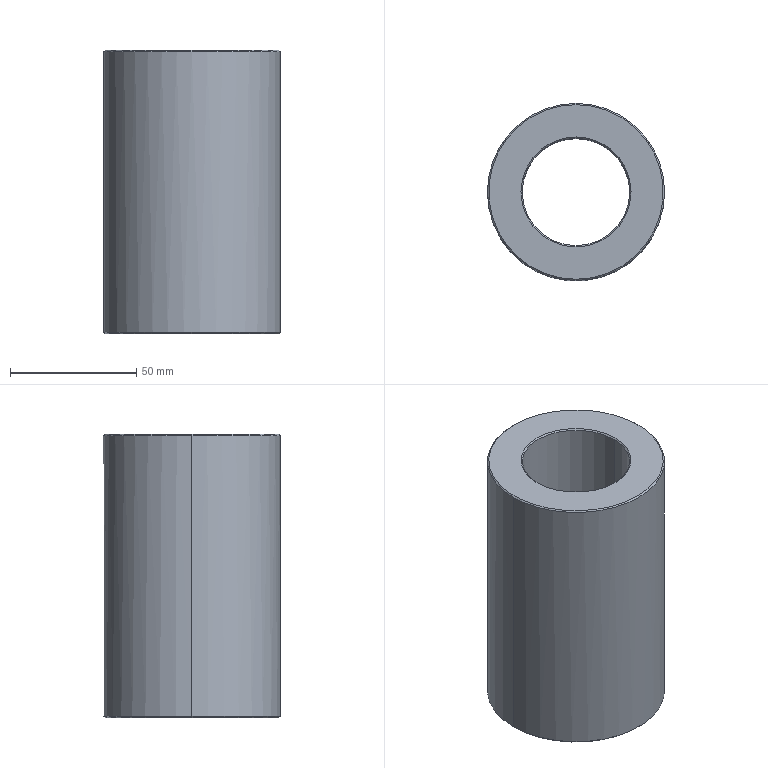Part | STEP file | Bearing sleeve_063_25.step_1 | 1 solid | 14 faces | box 70 x 70 x 112 mm | volume 272052 mm3 | cone 8 | cylinder 4 | plane 2 | commonest cylinder face diameters 42.5 x2 70 x2
STEP:
#1=CARTESIAN_POINT('',(0.,0.,0.));
#2=DIRECTION('',(0.,0.,1.));
#3=DIRECTION('',(1.,0.,0.));
#4=AXIS2_PLACEMENT_3D('',#1,#2,#3);
#5=CARTESIAN_POINT('',(35.,0.,-55.5));
#6=VERTEX_POINT('',#5);
#7=CARTESIAN_POINT('',(-35.,0.,-55.5));
#8=VERTEX_POINT('',#7);
#9=CARTESIAN_POINT('',(0.,0.,-55.5));
#10=DIRECTION('',(0.,0.,1.));
#11=DIRECTION('',(1.,0.,0.));
#12=AXIS2_PLACEMENT_3D('',#9,#10,#11);
#13=CIRCLE('',#12,35.);
#14=CARTESIAN_POINT('',(0.,0.,96.873));
#15=DIRECTION('',(0.,0.,1.));
#16=DIRECTION('',(1.,0.,0.));
#17=AXIS2_PLACEMENT_3D('',#14,#15,#16);
#18=CYLINDRICAL_SURFACE('',#17,35.);
#19=CARTESIAN_POINT('',(0.,-152.373));
#20=DIRECTION('',(1.,0.));
#21=VECTOR('',#20,1.);
#22=LINE('',#19,#21);
#23=(GEOMETRIC_REPRESENTATION_CONTEXT(2)PARAMETRIC_REPRESENTATION_CONTEXT()REPRESENTATION_CONTEXT('',''));
#24=DEFINITIONAL_REPRESENTATION('',(#22),#23);
#25=PCURVE('',#18,#24);
#26=CARTESIAN_POINT('',(0.,0.,-55.5));
#27=DIRECTION('',(0.,0.,1.));
#28=DIRECTION('',(1.,0.,0.));
#29=AXIS2_PLACEMENT_3D('',#26,#27,#28);
#30=CONICAL_SURFACE('',#29,35.,0.7854);
#31=CARTESIAN_POINT('',(0.,0.));
#32=DIRECTION('',(1.,0.));
#33=VECTOR('',#32,1.);
#34=LINE('',#31,#33);
#35=(GEOMETRIC_REPRESENTATION_CONTEXT(2)PARAMETRIC_REPRESENTATION_CONTEXT()REPRESENTATION_CONTEXT('',''));
#36=DEFINITIONAL_REPRESENTATION('',(#34),#35);
#37=PCURVE('',#30,#36);
#38=SURFACE_CURVE('',#13,(#25,#37),.PCURVE_S1.);
#39=EDGE_CURVE('',#6,#8,#38,.T.);
#40=ORIENTED_EDGE('',*,*,#39,.T.);
#41=CARTESIAN_POINT('',(-35.,0.,55.5));
#42=VERTEX_POINT('',#41);
#43=CARTESIAN_POINT('',(-35.,0.,96.873));
#44=DIRECTION('',(0.,0.,1.));
#45=VECTOR('',#44,1.);
#46=LINE('',#43,#45);
#47=CARTESIAN_POINT('',(3.142,0.));
#48=DIRECTION('',(0.,1.));
#49=VECTOR('',#48,1.);
#50=LINE('',#47,#49);
#51=(GEOMETRIC_REPRESENTATION_CONTEXT(2)PARAMETRIC_REPRESENTATION_CONTEXT()REPRESENTATION_CONTEXT('',''));
#52=DEFINITIONAL_REPRESENTATION('',(#50),#51);
#53=PCURVE('',#18,#52);
#54=CARTESIAN_POINT('',(0.,0.,96.873));
#55=DIRECTION('',(0.,0.,1.));
#56=DIRECTION('',(1.,0.,0.));
#57=AXIS2_PLACEMENT_3D('',#54,#55,#56);
#58=CYLINDRICAL_SURFACE('',#57,35.);
#59=CARTESIAN_POINT('',(3.142,0.));
#60=DIRECTION('',(0.,1.));
#61=VECTOR('',#60,1.);
#62=LINE('',#59,#61);
#63=(GEOMETRIC_REPRESENTATION_CONTEXT(2)PARAMETRIC_REPRESENTATION_CONTEXT()REPRESENTATION_CONTEXT('',''));
#64=DEFINITIONAL_REPRESENTATION('',(#62),#63);
#65=PCURVE('',#58,#64);
#66=SURFACE_CURVE('',#46,(#53,#65),.PCURVE_S1.);
#67=EDGE_CURVE('',#8,#42,#66,.T.);
#68=ORIENTED_EDGE('',*,*,#67,.T.);
#69=CARTESIAN_POINT('',(0.,35.,55.5));
#70=VERTEX_POINT('',#69);
#71=CARTESIAN_POINT('',(0.,0.,55.5));
#72=DIRECTION('',(0.,0.,-1.));
#73=DIRECTION('',(1.,0.,0.));
#74=AXIS2_PLACEMENT_3D('',#71,#72,#73);
#75=CIRCLE('',#74,35.);
#76=CARTESIAN_POINT('',(6.283,-41.373));
#77=DIRECTION('',(-1.,0.));
#78=VECTOR('',#77,1.);
#79=LINE('',#76,#78);
#80=(GEOMETRIC_REPRESENTATION_CONTEXT(2)PARAMETRIC_REPRESENTATION_CONTEXT()REPRESENTATION_CONTEXT('',''));
#81=DEFINITIONAL_REPRESENTATION('',(#79),#80);
#82=PCURVE('',#18,#81);
#83=CARTESIAN_POINT('',(0.,0.,55.5));
#84=DIRECTION('',(0.,0.,-1.));
#85=DIRECTION('',(0.,1.,0.));
#86=AXIS2_PLACEMENT_3D('',#83,#84,#85);
#87=CONICAL_SURFACE('',#86,35.,0.7854);
#88=CARTESIAN_POINT('',(1.571,0.));
#89=DIRECTION('',(1.,0.));
#90=VECTOR('',#89,1.);
#91=LINE('',#88,#90);
#92=(GEOMETRIC_REPRESENTATION_CONTEXT(2)PARAMETRIC_REPRESENTATION_CONTEXT()REPRESENTATION_CONTEXT('',''));
#93=DEFINITIONAL_REPRESENTATION('',(#91),#92);
#94=PCURVE('',#87,#93);
#95=SURFACE_CURVE('',#75,(#82,#94),.PCURVE_S1.);
#96=EDGE_CURVE('',#42,#70,#95,.T.);
#97=ORIENTED_EDGE('',*,*,#96,.T.);
#98=CARTESIAN_POINT('',(35.,0.,55.5));
#99=VERTEX_POINT('',#98);
#100=CARTESIAN_POINT('',(0.,0.,55.5));
#101=DIRECTION('',(0.,0.,-1.));
#102=DIRECTION('',(1.,0.,0.));
#103=AXIS2_PLACEMENT_3D('',#100,#101,#102);
#104=CIRCLE('',#103,35.);
#105=CARTESIAN_POINT('',(6.283,-41.373));
#106=DIRECTION('',(-1.,0.));
#107=VECTOR('',#106,1.);
#108=LINE('',#105,#107);
#109=(GEOMETRIC_REPRESENTATION_CONTEXT(2)PARAMETRIC_REPRESENTATION_CONTEXT()REPRESENTATION_CONTEXT('',''));
#110=DEFINITIONAL_REPRESENTATION('',(#108),#109);
#111=PCURVE('',#18,#110);
#112=CARTESIAN_POINT('',(0.,0.,55.5));
#113=DIRECTION('',(0.,0.,-1.));
#114=DIRECTION('',(0.,1.,0.));
#115=AXIS2_PLACEMENT_3D('',#112,#113,#114);
#116=CONICAL_SURFACE('',#115,35.,0.7854);
#117=CARTESIAN_POINT('',(-4.712,0.));
#118=DIRECTION('',(1.,0.));
#119=VECTOR('',#118,1.);
#120=LINE('',#117,#119);
#121=(GEOMETRIC_REPRESENTATION_CONTEXT(2)PARAMETRIC_REPRESENTATION_CONTEXT()REPRESENTATION_CONTEXT('',''));
#122=DEFINITIONAL_REPRESENTATION('',(#120),#121);
#123=PCURVE('',#116,#122);
#124=SURFACE_CURVE('',#104,(#111,#123),.PCURVE_S1.);
#125=EDGE_CURVE('',#70,#99,#124,.T.);
#126=ORIENTED_EDGE('',*,*,#125,.T.);
#127=CARTESIAN_POINT('',(35.,0.,96.873));
#128=DIRECTION('',(0.,0.,1.));
#129=VECTOR('',#128,1.);
#130=LINE('',#127,#129);
#131=CARTESIAN_POINT('',(0.,0.));
#132=DIRECTION('',(0.,1.));
#133=VECTOR('',#132,1.);
#134=LINE('',#131,#133);
#135=(GEOMETRIC_REPRESENTATION_CONTEXT(2)PARAMETRIC_REPRESENTATION_CONTEXT()REPRESENTATION_CONTEXT('',''));
#136=DEFINITIONAL_REPRESENTATION('',(#134),#135);
#137=PCURVE('',#18,#136);
#138=CARTESIAN_POINT('',(6.283,0.));
#139=DIRECTION('',(0.,1.));
#140=VECTOR('',#139,1.);
#141=LINE('',#138,#140);
#142=(GEOMETRIC_REPRESENTATION_CONTEXT(2)PARAMETRIC_REPRESENTATION_CONTEXT()REPRESENTATION_CONTEXT('',''));
#143=DEFINITIONAL_REPRESENTATION('',(#141),#142);
#144=PCURVE('',#58,#143);
#145=SURFACE_CURVE('',#130,(#137,#144),.PCURVE_S1.);
#146=EDGE_CURVE('',#6,#99,#145,.T.);
#147=ORIENTED_EDGE('',*,*,#146,.F.);
#148=EDGE_LOOP('',(#40,#68,#97,#126,#147));
#149=FACE_BOUND('',#148,.T.);
#150=ADVANCED_FACE('',(#149),#18,.T.);
#151=CARTESIAN_POINT('',(0.,34.5,56.));
#152=VERTEX_POINT('',#151);
#153=CARTESIAN_POINT('',(0.,-34.5,56.));
#154=VERTEX_POINT('',#153);
#155=CARTESIAN_POINT('',(0.,0.,56.));
#156=DIRECTION('',(0.,0.,-1.));
#157=DIRECTION('',(0.,1.,0.));
#158=AXIS2_PLACEMENT_3D('',#155,#156,#157);
#159=CIRCLE('',#158,34.5);
#160=CARTESIAN_POINT('',(0.,-0.5));
#161=DIRECTION('',(1.,0.));
#162=VECTOR('',#161,1.);
#163=LINE('',#160,#162);
#164=(GEOMETRIC_REPRESENTATION_CONTEXT(2)PARAMETRIC_REPRESENTATION_CONTEXT()REPRESENTATION_CONTEXT('',''));
#165=DEFINITIONAL_REPRESENTATION('',(#163),#164);
#166=PCURVE('',#116,#165);
#167=CARTESIAN_POINT('',(0.,21.75,56.));
#168=DIRECTION('',(0.,0.,-1.));
#169=DIRECTION('',(-1.,0.,0.));
#170=AXIS2_PLACEMENT_3D('',#167,#168,#169);
#171=PLANE('',#170);
#172=CARTESIAN_POINT('',(0.,-21.75));
#173=DIRECTION('',(0.,1.));
#174=AXIS2_PLACEMENT_2D('',#172,#173);
#175=CIRCLE('',#174,34.5);
#176=(GEOMETRIC_REPRESENTATION_CONTEXT(2)PARAMETRIC_REPRESENTATION_CONTEXT()REPRESENTATION_CONTEXT('',''));
#177=DEFINITIONAL_REPRESENTATION('',(#175),#176);
#178=PCURVE('',#171,#177);
#179=SURFACE_CURVE('',#159,(#166,#178),.PCURVE_S1.);
#180=EDGE_CURVE('',#152,#154,#179,.T.);
#181=ORIENTED_EDGE('',*,*,#180,.T.);
#182=CARTESIAN_POINT('',(0.,-35.,55.5));
#183=VERTEX_POINT('',#182);
#184=CARTESIAN_POINT('',(0.,-35.,55.5));
#185=DIRECTION('',(0.,-0.7071,-0.7071));
#186=VECTOR('',#185,1.);
#187=LINE('',#184,#186);
#188=CARTESIAN_POINT('',(3.142,0.));
#189=DIRECTION('',(0.,1.));
#190=VECTOR('',#189,1.);
#191=LINE('',#188,#190);
#192=(GEOMETRIC_REPRESENTATION_CONTEXT(2)PARAMETRIC_REPRESENTATION_CONTEXT()REPRESENTATION_CONTEXT('',''));
#193=DEFINITIONAL_REPRESENTATION('',(#191),#192);
#194=PCURVE('',#116,#193);
#195=CARTESIAN_POINT('',(3.142,0.));
#196=DIRECTION('',(0.,1.));
#197=VECTOR('',#196,1.);
#198=LINE('',#195,#197);
#199=(GEOMETRIC_REPRESENTATION_CONTEXT(2)PARAMETRIC_REPRESENTATION_CONTEXT()REPRESENTATION_CONTEXT('',''));
#200=DEFINITIONAL_REPRESENTATION('',(#198),#199);
#201=PCURVE('',#87,#200);
#202=SURFACE_CURVE('',#187,(#194,#201),.PCURVE_S1.);
#203=EDGE_CURVE('',#154,#183,#202,.T.);
#204=ORIENTED_EDGE('',*,*,#203,.T.);
#205=CARTESIAN_POINT('',(0.,0.,55.5));
#206=DIRECTION('',(0.,0.,-1.));
#207=DIRECTION('',(1.,0.,0.));
#208=AXIS2_PLACEMENT_3D('',#205,#206,#207);
#209=CIRCLE('',#208,35.);
#210=CARTESIAN_POINT('',(1.571,0.));
#211=DIRECTION('',(1.,0.));
#212=VECTOR('',#211,1.);
#213=LINE('',#210,#212);
#214=(GEOMETRIC_REPRESENTATION_CONTEXT(2)PARAMETRIC_REPRESENTATION_CONTEXT()REPRESENTATION_CONTEXT('',''));
#215=DEFINITIONAL_REPRESENTATION('',(#213),#214);
#216=PCURVE('',#116,#215);
#217=CARTESIAN_POINT('',(6.283,-41.373));
#218=DIRECTION('',(-1.,0.));
#219=VECTOR('',#218,1.);
#220=LINE('',#217,#219);
#221=(GEOMETRIC_REPRESENTATION_CONTEXT(2)PARAMETRIC_REPRESENTATION_CONTEXT()REPRESENTATION_CONTEXT('',''));
#222=DEFINITIONAL_REPRESENTATION('',(#220),#221);
#223=PCURVE('',#58,#222);
#224=SURFACE_CURVE('',#209,(#216,#223),.PCURVE_S1.);
#225=EDGE_CURVE('',#99,#183,#224,.T.);
#226=ORIENTED_EDGE('',*,*,#225,.F.);
#227=ORIENTED_EDGE('',*,*,#125,.F.);
#228=CARTESIAN_POINT('',(0.,35.,55.5));
#229=DIRECTION('',(0.,0.7071,-0.7071));
#230=VECTOR('',#229,1.);
#231=LINE('',#228,#230);
#232=CARTESIAN_POINT('',(0.,0.));
#233=DIRECTION('',(0.,1.));
#234=VECTOR('',#233,1.);
#235=LINE('',#232,#234);
#236=(GEOMETRIC_REPRESENTATION_CONTEXT(2)PARAMETRIC_REPRESENTATION_CONTEXT()REPRESENTATION_CONTEXT('',''));
#237=DEFINITIONAL_REPRESENTATION('',(#235),#236);
#238=PCURVE('',#116,#237);
#239=CARTESIAN_POINT('',(6.283,0.));
#240=DIRECTION('',(0.,1.));
#241=VECTOR('',#240,1.);
#242=LINE('',#239,#241);
#243=(GEOMETRIC_REPRESENTATION_CONTEXT(2)PARAMETRIC_REPRESENTATION_CONTEXT()REPRESENTATION_CONTEXT('',''));
#244=DEFINITIONAL_REPRESENTATION('',(#242),#243);
#245=PCURVE('',#87,#244);
#246=SURFACE_CURVE('',#231,(#238,#245),.PCURVE_S1.);
#247=EDGE_CURVE('',#152,#70,#246,.T.);
#248=ORIENTED_EDGE('',*,*,#247,.F.);
#249=EDGE_LOOP('',(#181,#204,#226,#227,#248));
#250=FACE_BOUND('',#249,.T.);
#251=ADVANCED_FACE('',(#250),#116,.T.);
#252=CARTESIAN_POINT('',(34.5,0.,-56.));
#253=VERTEX_POINT('',#252);
#254=CARTESIAN_POINT('',(-34.5,0.,-56.));
#255=VERTEX_POINT('',#254);
#256=CARTESIAN_POINT('',(0.,0.,-56.));
#257=DIRECTION('',(0.,0.,1.));
#258=DIRECTION('',(1.,0.,0.));
#259=AXIS2_PLACEMENT_3D('',#256,#257,#258);
#260=CIRCLE('',#259,34.5);
#261=CARTESIAN_POINT('',(0.,-0.5));
#262=DIRECTION('',(1.,0.));
#263=VECTOR('',#262,1.);
#264=LINE('',#261,#263);
#265=(GEOMETRIC_REPRESENTATION_CONTEXT(2)PARAMETRIC_REPRESENTATION_CONTEXT()REPRESENTATION_CONTEXT('',''));
#266=DEFINITIONAL_REPRESENTATION('',(#264),#265);
#267=PCURVE('',#30,#266);
#268=CARTESIAN_POINT('',(0.,34.5,-56.));
#269=DIRECTION('',(0.,0.,1.));
#270=DIRECTION('',(1.,0.,0.));
#271=AXIS2_PLACEMENT_3D('',#268,#269,#270);
#272=PLANE('',#271);
#273=CARTESIAN_POINT('',(0.,-34.5));
#274=DIRECTION('',(1.,0.));
#275=AXIS2_PLACEMENT_2D('',#273,#274);
#276=CIRCLE('',#275,34.5);
#277=(GEOMETRIC_REPRESENTATION_CONTEXT(2)PARAMETRIC_REPRESENTATION_CONTEXT()REPRESENTATION_CONTEXT('',''));
#278=DEFINITIONAL_REPRESENTATION('',(#276),#277);
#279=PCURVE('',#272,#278);
#280=SURFACE_CURVE('',#260,(#267,#279),.PCURVE_S1.);
#281=EDGE_CURVE('',#253,#255,#280,.T.);
#282=ORIENTED_EDGE('',*,*,#281,.T.);
#283=CARTESIAN_POINT('',(-35.,0.,-55.5));
#284=DIRECTION('',(-0.7071,0.,0.7071));
#285=VECTOR('',#284,1.);
#286=LINE('',#283,#285);
#287=CARTESIAN_POINT('',(3.142,0.));
#288=DIRECTION('',(0.,1.));
#289=VECTOR('',#288,1.);
#290=LINE('',#287,#289);
#291=(GEOMETRIC_REPRESENTATION_CONTEXT(2)PARAMETRIC_REPRESENTATION_CONTEXT()REPRESENTATION_CONTEXT('',''));
#292=DEFINITIONAL_REPRESENTATION('',(#290),#291);
#293=PCURVE('',#30,#292);
#294=CARTESIAN_POINT('',(0.,0.,-55.5));
#295=DIRECTION('',(0.,0.,1.));
#296=DIRECTION('',(1.,0.,0.));
#297=AXIS2_PLACEMENT_3D('',#294,#295,#296);
#298=CONICAL_SURFACE('',#297,35.,0.7854);
#299=CARTESIAN_POINT('',(3.142,0.));
#300=DIRECTION('',(0.,1.));
#301=VECTOR('',#300,1.);
#302=LINE('',#299,#301);
#303=(GEOMETRIC_REPRESENTATION_CONTEXT(2)PARAMETRIC_REPRESENTATION_CONTEXT()REPRESENTATION_CONTEXT('',''));
#304=DEFINITIONAL_REPRESENTATION('',(#302),#303);
#305=PCURVE('',#298,#304);
#306=SURFACE_CURVE('',#286,(#293,#305),.PCURVE_S1.);
#307=EDGE_CURVE('',#255,#8,#306,.T.);
#308=ORIENTED_EDGE('',*,*,#307,.T.);
#309=ORIENTED_EDGE('',*,*,#39,.F.);
#310=CARTESIAN_POINT('',(35.,0.,-55.5));
#311=DIRECTION('',(0.7071,0.,0.7071));
#312=VECTOR('',#311,1.);
#313=LINE('',#310,#312);
#314=CARTESIAN_POINT('',(0.,0.));
#315=DIRECTION('',(0.,1.));
#316=VECTOR('',#315,1.);
#317=LINE('',#314,#316);
#318=(GEOMETRIC_REPRESENTATION_CONTEXT(2)PARAMETRIC_REPRESENTATION_CONTEXT()REPRESENTATION_CONTEXT('',''));
#319=DEFINITIONAL_REPRESENTATION('',(#317),#318);
#320=PCURVE('',#30,#319);
#321=CARTESIAN_POINT('',(6.283,0.));
#322=DIRECTION('',(0.,1.));
#323=VECTOR('',#322,1.);
#324=LINE('',#321,#323);
#325=(GEOMETRIC_REPRESENTATION_CONTEXT(2)PARAMETRIC_REPRESENTATION_CONTEXT()REPRESENTATION_CONTEXT('',''));
#326=DEFINITIONAL_REPRESENTATION('',(#324),#325);
#327=PCURVE('',#298,#326);
#328=SURFACE_CURVE('',#313,(#320,#327),.PCURVE_S1.);
#329=EDGE_CURVE('',#253,#6,#328,.T.);
#330=ORIENTED_EDGE('',*,*,#329,.F.);
#331=EDGE_LOOP('',(#282,#308,#309,#330));
#332=FACE_BOUND('',#331,.T.);
#333=ADVANCED_FACE('',(#332),#30,.T.);
#334=CARTESIAN_POINT('',(-21.25,0.,55.5));
#335=VERTEX_POINT('',#334);
#336=CARTESIAN_POINT('',(0.,-21.25,55.5));
#337=VERTEX_POINT('',#336);
#338=CARTESIAN_POINT('',(0.,0.,55.5));
#339=DIRECTION('',(0.,0.,1.));
#340=DIRECTION('',(1.,0.,0.));
#341=AXIS2_PLACEMENT_3D('',#338,#339,#340);
#342=CIRCLE('',#341,21.25);
#343=CARTESIAN_POINT('',(0.,0.,56.));
#344=DIRECTION('',(0.,0.,1.));
#345=DIRECTION('',(0.,-1.,0.));
#346=AXIS2_PLACEMENT_3D('',#343,#344,#345);
#347=CONICAL_SURFACE('',#346,21.75,0.7854);
#348=CARTESIAN_POINT('',(1.571,-0.5));
#349=DIRECTION('',(1.,0.));
#350=VECTOR('',#349,1.);
#351=LINE('',#348,#350);
#352=(GEOMETRIC_REPRESENTATION_CONTEXT(2)PARAMETRIC_REPRESENTATION_CONTEXT()REPRESENTATION_CONTEXT('',''));
#353=DEFINITIONAL_REPRESENTATION('',(#351),#352);
#354=PCURVE('',#347,#353);
#355=CARTESIAN_POINT('',(0.,0.,96.873));
#356=DIRECTION('',(0.,0.,1.));
#357=DIRECTION('',(1.,0.,0.));
#358=AXIS2_PLACEMENT_3D('',#355,#356,#357);
#359=CYLINDRICAL_SURFACE('',#358,21.25);
#360=CARTESIAN_POINT('',(0.,-41.373));
#361=DIRECTION('',(1.,0.));
#362=VECTOR('',#361,1.);
#363=LINE('',#360,#362);
#364=(GEOMETRIC_REPRESENTATION_CONTEXT(2)PARAMETRIC_REPRESENTATION_CONTEXT()REPRESENTATION_CONTEXT('',''));
#365=DEFINITIONAL_REPRESENTATION('',(#363),#364);
#366=PCURVE('',#359,#365);
#367=SURFACE_CURVE('',#342,(#354,#366),.PCURVE_S1.);
#368=EDGE_CURVE('',#335,#337,#367,.T.);
#369=ORIENTED_EDGE('',*,*,#368,.T.);
#370=CARTESIAN_POINT('',(0.,-21.75,56.));
#371=VERTEX_POINT('',#370);
#372=CARTESIAN_POINT('',(0.,-21.75,56.));
#373=DIRECTION('',(0.,-0.7071,0.7071));
#374=VECTOR('',#373,1.);
#375=LINE('',#372,#374);
#376=CARTESIAN_POINT('',(6.283,0.));
#377=DIRECTION('',(0.,1.));
#378=VECTOR('',#377,1.);
#379=LINE('',#376,#378);
#380=(GEOMETRIC_REPRESENTATION_CONTEXT(2)PARAMETRIC_REPRESENTATION_CONTEXT()REPRESENTATION_CONTEXT('',''));
#381=DEFINITIONAL_REPRESENTATION('',(#379),#380);
#382=PCURVE('',#347,#381);
#383=CARTESIAN_POINT('',(0.,0.,56.));
#384=DIRECTION('',(0.,0.,1.));
#385=DIRECTION('',(0.,-1.,0.));
#386=AXIS2_PLACEMENT_3D('',#383,#384,#385);
#387=CONICAL_SURFACE('',#386,21.75,0.7854);
#388=CARTESIAN_POINT('',(0.,0.));
#389=DIRECTION('',(0.,1.));
#390=VECTOR('',#389,1.);
#391=LINE('',#388,#390);
#392=(GEOMETRIC_REPRESENTATION_CONTEXT(2)PARAMETRIC_REPRESENTATION_CONTEXT()REPRESENTATION_CONTEXT('',''));
#393=DEFINITIONAL_REPRESENTATION('',(#391),#392);
#394=PCURVE('',#387,#393);
#395=SURFACE_CURVE('',#375,(#382,#394),.PCURVE_S1.);
#396=EDGE_CURVE('',#337,#371,#395,.T.);
#397=ORIENTED_EDGE('',*,*,#396,.T.);
#398=CARTESIAN_POINT('',(0.,21.75,56.));
#399=VERTEX_POINT('',#398);
#400=CARTESIAN_POINT('',(0.,0.,56.));
#401=DIRECTION('',(0.,0.,1.));
#402=DIRECTION('',(0.,-1.,0.));
#403=AXIS2_PLACEMENT_3D('',#400,#401,#402);
#404=CIRCLE('',#403,21.75);
#405=CARTESIAN_POINT('',(0.,0.));
#406=DIRECTION('',(1.,0.));
#407=VECTOR('',#406,1.);
#408=LINE('',#405,#407);
#409=(GEOMETRIC_REPRESENTATION_CONTEXT(2)PARAMETRIC_REPRESENTATION_CONTEXT()REPRESENTATION_CONTEXT('',''));
#410=DEFINITIONAL_REPRESENTATION('',(#408),#409);
#411=PCURVE('',#347,#410);
#412=CARTESIAN_POINT('',(0.,-43.5));
#413=CARTESIAN_POINT('',(-37.672,-43.5));
#414=CARTESIAN_POINT('',(-18.836,-10.875));
#415=CARTESIAN_POINT('',(0.,21.75));
#416=CARTESIAN_POINT('',(18.836,-10.875));
#417=CARTESIAN_POINT('',(37.672,-43.5));
#418=CARTESIAN_POINT('',(0.,-43.5));
#419=(BOUNDED_CURVE()B_SPLINE_CURVE(2,(#412,#413,#414,#415,#416,#417,#418),.UNSPECIFIED.,.T.,.F.)B_SPLINE_CURVE_WITH_KNOTS((1,2,2,2,2,1),(-2.094,0.,2.094,4.189,6.283,8.378),.UNSPECIFIED.)CURVE()GEOMETRIC_REPRESENTATION_ITEM()RATIONAL_B_SPLINE_CURVE((1.,0.5,1.,0.5,1.,0.5,1.))REPRESENTATION_ITEM(''));
#420=(GEOMETRIC_REPRESENTATION_CONTEXT(2)PARAMETRIC_REPRESENTATION_CONTEXT()REPRESENTATION_CONTEXT('',''));
#421=DEFINITIONAL_REPRESENTATION('',(#419),#420);
#422=PCURVE('',#171,#421);
#423=SURFACE_CURVE('',#404,(#411,#422),.PCURVE_S1.);
#424=EDGE_CURVE('',#399,#371,#423,.T.);
#425=ORIENTED_EDGE('',*,*,#424,.F.);
#426=CARTESIAN_POINT('',(0.,21.25,55.5));
#427=VERTEX_POINT('',#426);
#428=CARTESIAN_POINT('',(0.,21.75,56.));
#429=DIRECTION('',(0.,0.7071,0.7071));
#430=VECTOR('',#429,1.);
#431=LINE('',#428,#430);
#432=CARTESIAN_POINT('',(3.142,0.));
#433=DIRECTION('',(0.,1.));
#434=VECTOR('',#433,1.);
#435=LINE('',#432,#434);
#436=(GEOMETRIC_REPRESENTATION_CONTEXT(2)PARAMETRIC_REPRESENTATION_CONTEXT()REPRESENTATION_CONTEXT('',''));
#437=DEFINITIONAL_REPRESENTATION('',(#435),#436);
#438=PCURVE('',#347,#437);
#439=CARTESIAN_POINT('',(3.142,0.));
#440=DIRECTION('',(0.,1.));
#441=VECTOR('',#440,1.);
#442=LINE('',#439,#441);
#443=(GEOMETRIC_REPRESENTATION_CONTEXT(2)PARAMETRIC_REPRESENTATION_CONTEXT()REPRESENTATION_CONTEXT('',''));
#444=DEFINITIONAL_REPRESENTATION('',(#442),#443);
#445=PCURVE('',#387,#444);
#446=SURFACE_CURVE('',#431,(#438,#445),.PCURVE_S1.);
#447=EDGE_CURVE('',#427,#399,#446,.T.);
#448=ORIENTED_EDGE('',*,*,#447,.F.);
#449=CARTESIAN_POINT('',(0.,0.,55.5));
#450=DIRECTION('',(0.,0.,1.));
#451=DIRECTION('',(1.,0.,0.));
#452=AXIS2_PLACEMENT_3D('',#449,#450,#451);
#453=CIRCLE('',#452,21.25);
#454=CARTESIAN_POINT('',(1.571,-0.5));
#455=DIRECTION('',(1.,0.));
#456=VECTOR('',#455,1.);
#457=LINE('',#454,#456);
#458=(GEOMETRIC_REPRESENTATION_CONTEXT(2)PARAMETRIC_REPRESENTATION_CONTEXT()REPRESENTATION_CONTEXT('',''));
#459=DEFINITIONAL_REPRESENTATION('',(#457),#458);
#460=PCURVE('',#347,#459);
#461=CARTESIAN_POINT('',(0.,0.,96.873));
#462=DIRECTION('',(0.,0.,1.));
#463=DIRECTION('',(1.,0.,0.));
#464=AXIS2_PLACEMENT_3D('',#461,#462,#463);
#465=CYLINDRICAL_SURFACE('',#464,21.25);
#466=CARTESIAN_POINT('',(0.,-41.373));
#467=DIRECTION('',(1.,0.));
#468=VECTOR('',#467,1.);
#469=LINE('',#466,#468);
#470=(GEOMETRIC_REPRESENTATION_CONTEXT(2)PARAMETRIC_REPRESENTATION_CONTEXT()REPRESENTATION_CONTEXT('',''));
#471=DEFINITIONAL_REPRESENTATION('',(#469),#470);
#472=PCURVE('',#465,#471);
#473=SURFACE_CURVE('',#453,(#460,#472),.PCURVE_S1.);
#474=EDGE_CURVE('',#427,#335,#473,.T.);
#475=ORIENTED_EDGE('',*,*,#474,.T.);
#476=EDGE_LOOP('',(#369,#397,#425,#448,#475));
#477=FACE_BOUND('',#476,.F.);
#478=ADVANCED_FACE('',(#477),#347,.F.);
#479=CARTESIAN_POINT('',(-21.25,0.,-55.5));
#480=VERTEX_POINT('',#479);
#481=CARTESIAN_POINT('',(-21.75,0.,-56.));
#482=VERTEX_POINT('',#481);
#483=CARTESIAN_POINT('',(-21.75,0.,-56.));
#484=DIRECTION('',(-0.7071,0.,-0.7071));
#485=VECTOR('',#484,1.);
#486=LINE('',#483,#485);
#487=CARTESIAN_POINT('',(0.,0.,-56.));
#488=DIRECTION('',(0.,0.,-1.));
#489=DIRECTION('',(-1.,0.,0.));
#490=AXIS2_PLACEMENT_3D('',#487,#488,#489);
#491=CONICAL_SURFACE('',#490,21.75,0.7854);
#492=CARTESIAN_POINT('',(6.283,0.));
#493=DIRECTION('',(0.,1.));
#494=VECTOR('',#493,1.);
#495=LINE('',#492,#494);
#496=(GEOMETRIC_REPRESENTATION_CONTEXT(2)PARAMETRIC_REPRESENTATION_CONTEXT()REPRESENTATION_CONTEXT('',''));
#497=DEFINITIONAL_REPRESENTATION('',(#495),#496);
#498=PCURVE('',#491,#497);
#499=CARTESIAN_POINT('',(0.,0.,-56.));
#500=DIRECTION('',(0.,0.,-1.));
#501=DIRECTION('',(-1.,0.,0.));
#502=AXIS2_PLACEMENT_3D('',#499,#500,#501);
#503=CONICAL_SURFACE('',#502,21.75,0.7854);
#504=CARTESIAN_POINT('',(0.,0.));
#505=DIRECTION('',(0.,1.));
#506=VECTOR('',#505,1.);
#507=LINE('',#504,#506);
#508=(GEOMETRIC_REPRESENTATION_CONTEXT(2)PARAMETRIC_REPRESENTATION_CONTEXT()REPRESENTATION_CONTEXT('',''));
#509=DEFINITIONAL_REPRESENTATION('',(#507),#508);
#510=PCURVE('',#503,#509);
#511=SURFACE_CURVE('',#486,(#498,#510),.PCURVE_S1.);
#512=EDGE_CURVE('',#480,#482,#511,.T.);
#513=ORIENTED_EDGE('',*,*,#512,.T.);
#514=CARTESIAN_POINT('',(21.75,0.,-56.));
#515=VERTEX_POINT('',#514);
#516=CARTESIAN_POINT('',(0.,0.,-56.));
#517=DIRECTION('',(0.,0.,-1.));
#518=DIRECTION('',(-1.,0.,0.));
#519=AXIS2_PLACEMENT_3D('',#516,#517,#518);
#520=CIRCLE('',#519,21.75);
#521=CARTESIAN_POINT('',(0.,0.));
#522=DIRECTION('',(1.,0.));
#523=VECTOR('',#522,1.);
#524=LINE('',#521,#523);
#525=(GEOMETRIC_REPRESENTATION_CONTEXT(2)PARAMETRIC_REPRESENTATION_CONTEXT()REPRESENTATION_CONTEXT('',''));
#526=DEFINITIONAL_REPRESENTATION('',(#524),#525);
#527=PCURVE('',#491,#526);
#528=CARTESIAN_POINT('',(-21.75,-34.5));
#529=CARTESIAN_POINT('',(-21.75,3.172));
#530=CARTESIAN_POINT('',(10.875,-15.664));
#531=CARTESIAN_POINT('',(43.5,-34.5));
#532=CARTESIAN_POINT('',(10.875,-53.336));
#533=CARTESIAN_POINT('',(-21.75,-72.172));
#534=CARTESIAN_POINT('',(-21.75,-34.5));
#535=(BOUNDED_CURVE()B_SPLINE_CURVE(2,(#528,#529,#530,#531,#532,#533,#534),.UNSPECIFIED.,.T.,.F.)B_SPLINE_CURVE_WITH_KNOTS((1,2,2,2,2,1),(-2.094,0.,2.094,4.189,6.283,8.378),.UNSPECIFIED.)CURVE()GEOMETRIC_REPRESENTATION_ITEM()RATIONAL_B_SPLINE_CURVE((1.,0.5,1.,0.5,1.,0.5,1.))REPRESENTATION_ITEM(''));
#536=(GEOMETRIC_REPRESENTATION_CONTEXT(2)PARAMETRIC_REPRESENTATION_CONTEXT()REPRESENTATION_CONTEXT('',''));
#537=DEFINITIONAL_REPRESENTATION('',(#535),#536);
#538=PCURVE('',#272,#537);
#539=SURFACE_CURVE('',#520,(#527,#538),.PCURVE_S1.);
#540=EDGE_CURVE('',#515,#482,#539,.T.);
#541=ORIENTED_EDGE('',*,*,#540,.F.);
#542=CARTESIAN_POINT('',(21.25,0.,-55.5));
#543=VERTEX_POINT('',#542);
#544=CARTESIAN_POINT('',(21.75,0.,-56.));
#545=DIRECTION('',(0.7071,0.,-0.7071));
#546=VECTOR('',#545,1.);
#547=LINE('',#544,#546);
#548=CARTESIAN_POINT('',(3.142,0.));
#549=DIRECTION('',(0.,1.));
#550=VECTOR('',#549,1.);
#551=LINE('',#548,#550);
#552=(GEOMETRIC_REPRESENTATION_CONTEXT(2)PARAMETRIC_REPRESENTATION_CONTEXT()REPRESENTATION_CONTEXT('',''));
#553=DEFINITIONAL_REPRESENTATION('',(#551),#552);
#554=PCURVE('',#491,#553);
#555=CARTESIAN_POINT('',(3.142,0.));
#556=DIRECTION('',(0.,1.));
#557=VECTOR('',#556,1.);
#558=LINE('',#555,#557);
#559=(GEOMETRIC_REPRESENTATION_CONTEXT(2)PARAMETRIC_REPRESENTATION_CONTEXT()REPRESENTATION_CONTEXT('',''));
#560=DEFINITIONAL_REPRESENTATION('',(#558),#559);
#561=PCURVE('',#503,#560);
#562=SURFACE_CURVE('',#547,(#554,#561),.PCURVE_S1.);
#563=EDGE_CURVE('',#543,#515,#562,.T.);
#564=ORIENTED_EDGE('',*,*,#563,.F.);
#565=CARTESIAN_POINT('',(0.,0.,-55.5));
#566=DIRECTION('',(0.,0.,-1.));
#567=DIRECTION('',(-1.,0.,0.));
#568=AXIS2_PLACEMENT_3D('',#565,#566,#567);
#569=CIRCLE('',#568,21.25);
#570=CARTESIAN_POINT('',(0.,-0.5));
#571=DIRECTION('',(1.,0.));
#572=VECTOR('',#571,1.);
#573=LINE('',#570,#572);
#574=(GEOMETRIC_REPRESENTATION_CONTEXT(2)PARAMETRIC_REPRESENTATION_CONTEXT()REPRESENTATION_CONTEXT('',''));
#575=DEFINITIONAL_REPRESENTATION('',(#573),#574);
#576=PCURVE('',#491,#575);
#577=CARTESIAN_POINT('',(9.425,-152.373));
#578=DIRECTION('',(-1.,0.));
#579=VECTOR('',#578,1.);
#580=LINE('',#577,#579);
#581=(GEOMETRIC_REPRESENTATION_CONTEXT(2)PARAMETRIC_REPRESENTATION_CONTEXT()REPRESENTATION_CONTEXT('',''));
#582=DEFINITIONAL_REPRESENTATION('',(#580),#581);
#583=PCURVE('',#359,#582);
#584=SURFACE_CURVE('',#569,(#576,#583),.PCURVE_S1.);
#585=EDGE_CURVE('',#543,#480,#584,.T.);
#586=ORIENTED_EDGE('',*,*,#585,.T.);
#587=EDGE_LOOP('',(#513,#541,#564,#586));
#588=FACE_BOUND('',#587,.F.);
#589=ADVANCED_FACE('',(#588),#491,.F.);
#590=CARTESIAN_POINT('',(21.25,0.,55.5));
#591=VERTEX_POINT('',#590);
#592=CARTESIAN_POINT('',(21.25,0.,96.873));
#593=DIRECTION('',(0.,0.,1.));
#594=VECTOR('',#593,1.);
#595=LINE('',#592,#594);
#596=CARTESIAN_POINT('',(6.283,0.));
#597=DIRECTION('',(0.,1.));
#598=VECTOR('',#597,1.);
#599=LINE('',#596,#598);
#600=(GEOMETRIC_REPRESENTATION_CONTEXT(2)PARAMETRIC_REPRESENTATION_CONTEXT()REPRESENTATION_CONTEXT('',''));
#601=DEFINITIONAL_REPRESENTATION('',(#599),#600);
#602=PCURVE('',#359,#601);
#603=CARTESIAN_POINT('',(0.,0.));
#604=DIRECTION('',(0.,1.));
#605=VECTOR('',#604,1.);
#606=LINE('',#603,#605);
#607=(GEOMETRIC_REPRESENTATION_CONTEXT(2)PARAMETRIC_REPRESENTATION_CONTEXT()REPRESENTATION_CONTEXT('',''));
#608=DEFINITIONAL_REPRESENTATION('',(#606),#607);
#609=PCURVE('',#465,#608);
#610=SURFACE_CURVE('',#595,(#602,#609),.PCURVE_S1.);
#611=EDGE_CURVE('',#543,#591,#610,.T.);
#612=ORIENTED_EDGE('',*,*,#611,.T.);
#613=CARTESIAN_POINT('',(0.,0.,55.5));
#614=DIRECTION('',(0.,0.,1.));
#615=DIRECTION('',(1.,0.,0.));
#616=AXIS2_PLACEMENT_3D('',#613,#614,#615);
#617=CIRCLE('',#616,21.25);
#618=CARTESIAN_POINT('',(0.,-41.373));
#619=DIRECTION('',(1.,0.));
#620=VECTOR('',#619,1.);
#621=LINE('',#618,#620);
#622=(GEOMETRIC_REPRESENTATION_CONTEXT(2)PARAMETRIC_REPRESENTATION_CONTEXT()REPRESENTATION_CONTEXT('',''));
#623=DEFINITIONAL_REPRESENTATION('',(#621),#622);
#624=PCURVE('',#359,#623);
#625=CARTESIAN_POINT('',(-4.712,-0.5));
#626=DIRECTION('',(1.,0.));
#627=VECTOR('',#626,1.);
#628=LINE('',#625,#627);
#629=(GEOMETRIC_REPRESENTATION_CONTEXT(2)PARAMETRIC_REPRESENTATION_CONTEXT()REPRESENTATION_CONTEXT('',''));
#630=DEFINITIONAL_REPRESENTATION('',(#628),#629);
#631=PCURVE('',#387,#630);
#632=SURFACE_CURVE('',#617,(#624,#631),.PCURVE_S1.);
#633=EDGE_CURVE('',#337,#591,#632,.T.);
#634=ORIENTED_EDGE('',*,*,#633,.F.);
#635=ORIENTED_EDGE('',*,*,#368,.F.);
#636=CARTESIAN_POINT('',(-21.25,0.,96.873));
#637=DIRECTION('',(0.,0.,1.));
#638=VECTOR('',#637,1.);
#639=LINE('',#636,#638);
#640=CARTESIAN_POINT('',(3.142,0.));
#641=DIRECTION('',(0.,1.));
#642=VECTOR('',#641,1.);
#643=LINE('',#640,#642);
#644=(GEOMETRIC_REPRESENTATION_CONTEXT(2)PARAMETRIC_REPRESENTATION_CONTEXT()REPRESENTATION_CONTEXT('',''));
#645=DEFINITIONAL_REPRESENTATION('',(#643),#644);
#646=PCURVE('',#359,#645);
#647=CARTESIAN_POINT('',(3.142,0.));
#648=DIRECTION('',(0.,1.));
#649=VECTOR('',#648,1.);
#650=LINE('',#647,#649);
#651=(GEOMETRIC_REPRESENTATION_CONTEXT(2)PARAMETRIC_REPRESENTATION_CONTEXT()REPRESENTATION_CONTEXT('',''));
#652=DEFINITIONAL_REPRESENTATION('',(#650),#651);
#653=PCURVE('',#465,#652);
#654=SURFACE_CURVE('',#639,(#646,#653),.PCURVE_S1.);
#655=EDGE_CURVE('',#480,#335,#654,.T.);
#656=ORIENTED_EDGE('',*,*,#655,.F.);
#657=ORIENTED_EDGE('',*,*,#585,.F.);
#658=EDGE_LOOP('',(#612,#634,#635,#656,#657));
#659=FACE_BOUND('',#658,.F.);
#660=ADVANCED_FACE('',(#659),#359,.F.);
#661=ORIENTED_EDGE('',*,*,#67,.F.);
#662=CARTESIAN_POINT('',(0.,0.,-55.5));
#663=DIRECTION('',(0.,0.,1.));
#664=DIRECTION('',(1.,0.,0.));
#665=AXIS2_PLACEMENT_3D('',#662,#663,#664);
#666=CIRCLE('',#665,35.);
#667=CARTESIAN_POINT('',(0.,-152.373));
#668=DIRECTION('',(1.,0.));
#669=VECTOR('',#668,1.);
#670=LINE('',#667,#669);
#671=(GEOMETRIC_REPRESENTATION_CONTEXT(2)PARAMETRIC_REPRESENTATION_CONTEXT()REPRESENTATION_CONTEXT('',''));
#672=DEFINITIONAL_REPRESENTATION('',(#670),#671);
#673=PCURVE('',#58,#672);
#674=CARTESIAN_POINT('',(0.,0.));
#675=DIRECTION('',(1.,0.));
#676=VECTOR('',#675,1.);
#677=LINE('',#674,#676);
#678=(GEOMETRIC_REPRESENTATION_CONTEXT(2)PARAMETRIC_REPRESENTATION_CONTEXT()REPRESENTATION_CONTEXT('',''));
#679=DEFINITIONAL_REPRESENTATION('',(#677),#678);
#680=PCURVE('',#298,#679);
#681=SURFACE_CURVE('',#666,(#673,#680),.PCURVE_S1.);
#682=EDGE_CURVE('',#8,#6,#681,.T.);
#683=ORIENTED_EDGE('',*,*,#682,.T.);
#684=ORIENTED_EDGE('',*,*,#146,.T.);
#685=ORIENTED_EDGE('',*,*,#225,.T.);
#686=CARTESIAN_POINT('',(0.,0.,55.5));
#687=DIRECTION('',(0.,0.,-1.));
#688=DIRECTION('',(1.,0.,0.));
#689=AXIS2_PLACEMENT_3D('',#686,#687,#688);
#690=CIRCLE('',#689,35.);
#691=CARTESIAN_POINT('',(6.283,-41.373));
#692=DIRECTION('',(-1.,0.));
#693=VECTOR('',#692,1.);
#694=LINE('',#691,#693);
#695=(GEOMETRIC_REPRESENTATION_CONTEXT(2)PARAMETRIC_REPRESENTATION_CONTEXT()REPRESENTATION_CONTEXT('',''));
#696=DEFINITIONAL_REPRESENTATION('',(#694),#695);
#697=PCURVE('',#58,#696);
#698=CARTESIAN_POINT('',(1.571,0.));
#699=DIRECTION('',(1.,0.));
#700=VECTOR('',#699,1.);
#701=LINE('',#698,#700);
#702=(GEOMETRIC_REPRESENTATION_CONTEXT(2)PARAMETRIC_REPRESENTATION_CONTEXT()REPRESENTATION_CONTEXT('',''));
#703=DEFINITIONAL_REPRESENTATION('',(#701),#702);
#704=PCURVE('',#87,#703);
#705=SURFACE_CURVE('',#690,(#697,#704),.PCURVE_S1.);
#706=EDGE_CURVE('',#183,#42,#705,.T.);
#707=ORIENTED_EDGE('',*,*,#706,.T.);
#708=EDGE_LOOP('',(#661,#683,#684,#685,#707));
#709=FACE_BOUND('',#708,.T.);
#710=ADVANCED_FACE('',(#709),#58,.T.);
#711=ORIENTED_EDGE('',*,*,#203,.F.);
#712=CARTESIAN_POINT('',(0.,0.,56.));
#713=DIRECTION('',(0.,0.,-1.));
#714=DIRECTION('',(0.,1.,0.));
#715=AXIS2_PLACEMENT_3D('',#712,#713,#714);
#716=CIRCLE('',#715,34.5);
#717=CARTESIAN_POINT('',(0.,-0.5));
#718=DIRECTION('',(1.,0.));
#719=VECTOR('',#718,1.);
#720=LINE('',#717,#719);
#721=(GEOMETRIC_REPRESENTATION_CONTEXT(2)PARAMETRIC_REPRESENTATION_CONTEXT()REPRESENTATION_CONTEXT('',''));
#722=DEFINITIONAL_REPRESENTATION('',(#720),#721);
#723=PCURVE('',#87,#722);
#724=CARTESIAN_POINT('',(0.,-21.75));
#725=DIRECTION('',(0.,1.));
#726=AXIS2_PLACEMENT_2D('',#724,#725);
#727=CIRCLE('',#726,34.5);
#728=(GEOMETRIC_REPRESENTATION_CONTEXT(2)PARAMETRIC_REPRESENTATION_CONTEXT()REPRESENTATION_CONTEXT('',''));
#729=DEFINITIONAL_REPRESENTATION('',(#727),#728);
#730=PCURVE('',#171,#729);
#731=SURFACE_CURVE('',#716,(#723,#730),.PCURVE_S1.);
#732=EDGE_CURVE('',#154,#152,#731,.T.);
#733=ORIENTED_EDGE('',*,*,#732,.T.);
#734=ORIENTED_EDGE('',*,*,#247,.T.);
#735=ORIENTED_EDGE('',*,*,#96,.F.);
#736=ORIENTED_EDGE('',*,*,#706,.F.);
#737=EDGE_LOOP('',(#711,#733,#734,#735,#736));
#738=FACE_BOUND('',#737,.T.);
#739=ADVANCED_FACE('',(#738),#87,.T.);
#740=ORIENTED_EDGE('',*,*,#307,.F.);
#741=CARTESIAN_POINT('',(0.,0.,-56.));
#742=DIRECTION('',(0.,0.,1.));
#743=DIRECTION('',(1.,0.,0.));
#744=AXIS2_PLACEMENT_3D('',#741,#742,#743);
#745=CIRCLE('',#744,34.5);
#746=CARTESIAN_POINT('',(0.,-0.5));
#747=DIRECTION('',(1.,0.));
#748=VECTOR('',#747,1.);
#749=LINE('',#746,#748);
#750=(GEOMETRIC_REPRESENTATION_CONTEXT(2)PARAMETRIC_REPRESENTATION_CONTEXT()REPRESENTATION_CONTEXT('',''));
#751=DEFINITIONAL_REPRESENTATION('',(#749),#750);
#752=PCURVE('',#298,#751);
#753=CARTESIAN_POINT('',(0.,-34.5));
#754=DIRECTION('',(1.,0.));
#755=AXIS2_PLACEMENT_2D('',#753,#754);
#756=CIRCLE('',#755,34.5);
#757=(GEOMETRIC_REPRESENTATION_CONTEXT(2)PARAMETRIC_REPRESENTATION_CONTEXT()REPRESENTATION_CONTEXT('',''));
#758=DEFINITIONAL_REPRESENTATION('',(#756),#757);
#759=PCURVE('',#272,#758);
#760=SURFACE_CURVE('',#745,(#752,#759),.PCURVE_S1.);
#761=EDGE_CURVE('',#255,#253,#760,.T.);
#762=ORIENTED_EDGE('',*,*,#761,.T.);
#763=ORIENTED_EDGE('',*,*,#329,.T.);
#764=ORIENTED_EDGE('',*,*,#682,.F.);
#765=EDGE_LOOP('',(#740,#762,#763,#764));
#766=FACE_BOUND('',#765,.T.);
#767=ADVANCED_FACE('',(#766),#298,.T.);
#768=ORIENTED_EDGE('',*,*,#180,.F.);
#769=ORIENTED_EDGE('',*,*,#732,.F.);
#770=EDGE_LOOP('',(#768,#769));
#771=FACE_BOUND('',#770,.T.);
#772=CARTESIAN_POINT('',(0.,0.,56.));
#773=DIRECTION('',(0.,0.,1.));
#774=DIRECTION('',(0.,-1.,0.));
#775=AXIS2_PLACEMENT_3D('',#772,#773,#774);
#776=CIRCLE('',#775,21.75);
#777=CARTESIAN_POINT('',(0.,-43.5));
#778=CARTESIAN_POINT('',(-37.672,-43.5));
#779=CARTESIAN_POINT('',(-18.836,-10.875));
#780=CARTESIAN_POINT('',(0.,21.75));
#781=CARTESIAN_POINT('',(18.836,-10.875));
#782=CARTESIAN_POINT('',(37.672,-43.5));
#783=CARTESIAN_POINT('',(0.,-43.5));
#784=(BOUNDED_CURVE()B_SPLINE_CURVE(2,(#777,#778,#779,#780,#781,#782,#783),.UNSPECIFIED.,.T.,.F.)B_SPLINE_CURVE_WITH_KNOTS((1,2,2,2,2,1),(-2.094,0.,2.094,4.189,6.283,8.378),.UNSPECIFIED.)CURVE()GEOMETRIC_REPRESENTATION_ITEM()RATIONAL_B_SPLINE_CURVE((1.,0.5,1.,0.5,1.,0.5,1.))REPRESENTATION_ITEM(''));
#785=(GEOMETRIC_REPRESENTATION_CONTEXT(2)PARAMETRIC_REPRESENTATION_CONTEXT()REPRESENTATION_CONTEXT('',''));
#786=DEFINITIONAL_REPRESENTATION('',(#784),#785);
#787=PCURVE('',#171,#786);
#788=CARTESIAN_POINT('',(0.,0.));
#789=DIRECTION('',(1.,0.));
#790=VECTOR('',#789,1.);
#791=LINE('',#788,#790);
#792=(GEOMETRIC_REPRESENTATION_CONTEXT(2)PARAMETRIC_REPRESENTATION_CONTEXT()REPRESENTATION_CONTEXT('',''));
#793=DEFINITIONAL_REPRESENTATION('',(#791),#792);
#794=PCURVE('',#387,#793);
#795=SURFACE_CURVE('',#776,(#787,#794),.PCURVE_S1.);
#796=EDGE_CURVE('',#371,#399,#795,.T.);
#797=ORIENTED_EDGE('',*,*,#796,.F.);
#798=ORIENTED_EDGE('',*,*,#424,.F.);
#799=EDGE_LOOP('',(#797,#798));
#800=FACE_BOUND('',#799,.T.);
#801=ADVANCED_FACE('',(#771,#800),#171,.F.);
#802=CARTESIAN_POINT('',(0.,0.,-56.));
#803=DIRECTION('',(0.,0.,-1.));
#804=DIRECTION('',(-1.,0.,0.));
#805=AXIS2_PLACEMENT_3D('',#802,#803,#804);
#806=CIRCLE('',#805,21.75);
#807=CARTESIAN_POINT('',(-21.75,-34.5));
#808=CARTESIAN_POINT('',(-21.75,3.172));
#809=CARTESIAN_POINT('',(10.875,-15.664));
#810=CARTESIAN_POINT('',(43.5,-34.5));
#811=CARTESIAN_POINT('',(10.875,-53.336));
#812=CARTESIAN_POINT('',(-21.75,-72.172));
#813=CARTESIAN_POINT('',(-21.75,-34.5));
#814=(BOUNDED_CURVE()B_SPLINE_CURVE(2,(#807,#808,#809,#810,#811,#812,#813),.UNSPECIFIED.,.T.,.F.)B_SPLINE_CURVE_WITH_KNOTS((1,2,2,2,2,1),(-2.094,0.,2.094,4.189,6.283,8.378),.UNSPECIFIED.)CURVE()GEOMETRIC_REPRESENTATION_ITEM()RATIONAL_B_SPLINE_CURVE((1.,0.5,1.,0.5,1.,0.5,1.))REPRESENTATION_ITEM(''));
#815=(GEOMETRIC_REPRESENTATION_CONTEXT(2)PARAMETRIC_REPRESENTATION_CONTEXT()REPRESENTATION_CONTEXT('',''));
#816=DEFINITIONAL_REPRESENTATION('',(#814),#815);
#817=PCURVE('',#272,#816);
#818=CARTESIAN_POINT('',(0.,0.));
#819=DIRECTION('',(1.,0.));
#820=VECTOR('',#819,1.);
#821=LINE('',#818,#820);
#822=(GEOMETRIC_REPRESENTATION_CONTEXT(2)PARAMETRIC_REPRESENTATION_CONTEXT()REPRESENTATION_CONTEXT('',''));
#823=DEFINITIONAL_REPRESENTATION('',(#821),#822);
#824=PCURVE('',#503,#823);
#825=SURFACE_CURVE('',#806,(#817,#824),.PCURVE_S1.);
#826=EDGE_CURVE('',#482,#515,#825,.T.);
#827=ORIENTED_EDGE('',*,*,#826,.F.);
#828=ORIENTED_EDGE('',*,*,#540,.F.);
#829=EDGE_LOOP('',(#827,#828));
#830=FACE_BOUND('',#829,.T.);
#831=ORIENTED_EDGE('',*,*,#281,.F.);
#832=ORIENTED_EDGE('',*,*,#761,.F.);
#833=EDGE_LOOP('',(#831,#832));
#834=FACE_BOUND('',#833,.T.);
#835=ADVANCED_FACE('',(#830,#834),#272,.F.);
#836=ORIENTED_EDGE('',*,*,#796,.F.);
#837=ORIENTED_EDGE('',*,*,#396,.F.);
#838=ORIENTED_EDGE('',*,*,#633,.T.);
#839=CARTESIAN_POINT('',(0.,0.,55.5));
#840=DIRECTION('',(0.,0.,1.));
#841=DIRECTION('',(1.,0.,0.));
#842=AXIS2_PLACEMENT_3D('',#839,#840,#841);
#843=CIRCLE('',#842,21.25);
#844=CARTESIAN_POINT('',(1.571,-0.5));
#845=DIRECTION('',(1.,0.));
#846=VECTOR('',#845,1.);
#847=LINE('',#844,#846);
#848=(GEOMETRIC_REPRESENTATION_CONTEXT(2)PARAMETRIC_REPRESENTATION_CONTEXT()REPRESENTATION_CONTEXT('',''));
#849=DEFINITIONAL_REPRESENTATION('',(#847),#848);
#850=PCURVE('',#387,#849);
#851=CARTESIAN_POINT('',(0.,-41.373));
#852=DIRECTION('',(1.,0.));
#853=VECTOR('',#852,1.);
#854=LINE('',#851,#853);
#855=(GEOMETRIC_REPRESENTATION_CONTEXT(2)PARAMETRIC_REPRESENTATION_CONTEXT()REPRESENTATION_CONTEXT('',''));
#856=DEFINITIONAL_REPRESENTATION('',(#854),#855);
#857=PCURVE('',#465,#856);
#858=SURFACE_CURVE('',#843,(#850,#857),.PCURVE_S1.);
#859=EDGE_CURVE('',#591,#427,#858,.T.);
#860=ORIENTED_EDGE('',*,*,#859,.T.);
#861=ORIENTED_EDGE('',*,*,#447,.T.);
#862=EDGE_LOOP('',(#836,#837,#838,#860,#861));
#863=FACE_BOUND('',#862,.F.);
#864=ADVANCED_FACE('',(#863),#387,.F.);
#865=ORIENTED_EDGE('',*,*,#826,.F.);
#866=ORIENTED_EDGE('',*,*,#512,.F.);
#867=CARTESIAN_POINT('',(0.,0.,-55.5));
#868=DIRECTION('',(0.,0.,-1.));
#869=DIRECTION('',(-1.,0.,0.));
#870=AXIS2_PLACEMENT_3D('',#867,#868,#869);
#871=CIRCLE('',#870,21.25);
#872=CARTESIAN_POINT('',(0.,-0.5));
#873=DIRECTION('',(1.,0.));
#874=VECTOR('',#873,1.);
#875=LINE('',#872,#874);
#876=(GEOMETRIC_REPRESENTATION_CONTEXT(2)PARAMETRIC_REPRESENTATION_CONTEXT()REPRESENTATION_CONTEXT('',''));
#877=DEFINITIONAL_REPRESENTATION('',(#875),#876);
#878=PCURVE('',#503,#877);
#879=CARTESIAN_POINT('',(3.142,-152.373));
#880=DIRECTION('',(-1.,0.));
#881=VECTOR('',#880,1.);
#882=LINE('',#879,#881);
#883=(GEOMETRIC_REPRESENTATION_CONTEXT(2)PARAMETRIC_REPRESENTATION_CONTEXT()REPRESENTATION_CONTEXT('',''));
#884=DEFINITIONAL_REPRESENTATION('',(#882),#883);
#885=PCURVE('',#465,#884);
#886=SURFACE_CURVE('',#871,(#878,#885),.PCURVE_S1.);
#887=EDGE_CURVE('',#480,#543,#886,.T.);
#888=ORIENTED_EDGE('',*,*,#887,.T.);
#889=ORIENTED_EDGE('',*,*,#563,.T.);
#890=EDGE_LOOP('',(#865,#866,#888,#889));
#891=FACE_BOUND('',#890,.F.);
#892=ADVANCED_FACE('',(#891),#503,.F.);
#893=ORIENTED_EDGE('',*,*,#474,.F.);
#894=ORIENTED_EDGE('',*,*,#859,.F.);
#895=ORIENTED_EDGE('',*,*,#611,.F.);
#896=ORIENTED_EDGE('',*,*,#887,.F.);
#897=ORIENTED_EDGE('',*,*,#655,.T.);
#898=EDGE_LOOP('',(#893,#894,#895,#896,#897));
#899=FACE_BOUND('',#898,.F.);
#900=ADVANCED_FACE('',(#899),#465,.F.);
#901=CLOSED_SHELL('',(#150,#251,#333,#478,#589,#660,#710,#739,#767,#801,#835,#864,#892,#900));
#902=MANIFOLD_SOLID_BREP('',#901);
#903=(LENGTH_UNIT()NAMED_UNIT(*)SI_UNIT(.MILLI.,.METRE.));
#904=UNCERTAINTY_MEASURE_WITH_UNIT(LENGTH_MEASURE(0.0000001),#903,'','');
#905=(NAMED_UNIT(*)PLANE_ANGLE_UNIT()SI_UNIT($,.RADIAN.));
#906=(NAMED_UNIT(*)SI_UNIT($,.STERADIAN.)SOLID_ANGLE_UNIT());
#907=(GEOMETRIC_REPRESENTATION_CONTEXT(3)GLOBAL_UNCERTAINTY_ASSIGNED_CONTEXT((#904))GLOBAL_UNIT_ASSIGNED_CONTEXT((#903,#905,#906))REPRESENTATION_CONTEXT('',''));
#908=ADVANCED_BREP_SHAPE_REPRESENTATION('',(#4,#902),#907);